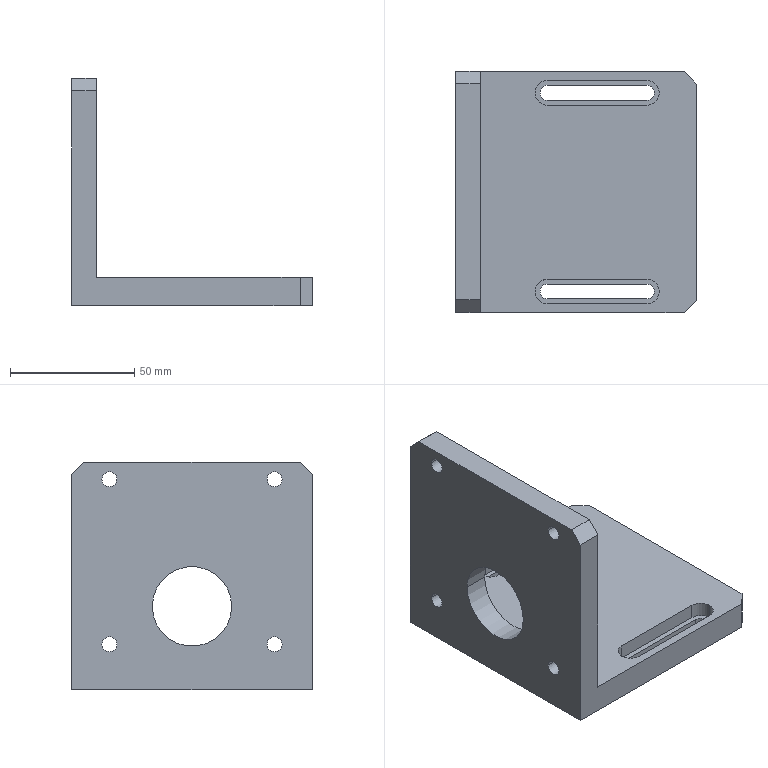Part | STEP file | Motor fixing bracket | 1 solid | 44 faces | box 97 x 97 x 91.5 mm | volume 167399 mm3 | cylinder 22 | plane 22 | commonest cylinder face diameters 6 x14 10 x6 32 x2
STEP:
#1=CARTESIAN_POINT('',(28.5,45.,5.5));
#2=VERTEX_POINT('',#1);
#3=CARTESIAN_POINT('',(33.5,40.,5.5));
#4=VERTEX_POINT('',#3);
#5=CARTESIAN_POINT('',(28.5,40.,5.5));
#6=DIRECTION('',(0.,0.,-1.));
#7=DIRECTION('',(1.,0.,0.));
#8=AXIS2_PLACEMENT_3D('',#5,#6,#7);
#9=CIRCLE('',#8,5.);
#10=EDGE_CURVE('',#2,#4,#9,.T.);
#11=ORIENTED_EDGE('',*,*,#10,.T.);
#12=CARTESIAN_POINT('',(33.5,40.,11.5));
#13=VERTEX_POINT('',#12);
#14=CARTESIAN_POINT('',(33.5,40.,5.5));
#15=DIRECTION('',(0.,0.,1.));
#16=VECTOR('',#15,1000.);
#17=LINE('',#14,#16);
#18=EDGE_CURVE('',#4,#13,#17,.T.);
#19=ORIENTED_EDGE('',*,*,#18,.T.);
#20=CARTESIAN_POINT('',(28.5,45.,11.5));
#21=VERTEX_POINT('',#20);
#22=CARTESIAN_POINT('',(28.5,40.,11.5));
#23=DIRECTION('',(0.,0.,-1.));
#24=DIRECTION('',(1.,0.,0.));
#25=AXIS2_PLACEMENT_3D('',#22,#23,#24);
#26=CIRCLE('',#25,5.);
#27=EDGE_CURVE('',#21,#13,#26,.T.);
#28=ORIENTED_EDGE('',*,*,#27,.F.);
#29=CARTESIAN_POINT('',(28.5,45.,5.5));
#30=DIRECTION('',(0.,0.,1.));
#31=VECTOR('',#30,1000.);
#32=LINE('',#29,#31);
#33=EDGE_CURVE('',#2,#21,#32,.T.);
#34=ORIENTED_EDGE('',*,*,#33,.F.);
#35=EDGE_LOOP('',(#11,#19,#28,#34));
#36=FACE_OUTER_BOUND('',#35,.T.);
#37=CARTESIAN_POINT('',(28.5,40.,5.5));
#38=DIRECTION('',(0.,0.,1.));
#39=DIRECTION('',(1.,0.,0.));
#40=AXIS2_PLACEMENT_3D('',#37,#38,#39);
#41=CYLINDRICAL_SURFACE('',#40,5.);
#42=ADVANCED_FACE('',(#36),#41,.F.);
#43=CARTESIAN_POINT('',(33.5,-40.,5.5));
#44=VERTEX_POINT('',#43);
#45=CARTESIAN_POINT('',(28.5,-35.,5.5));
#46=VERTEX_POINT('',#45);
#47=CARTESIAN_POINT('',(28.5,-40.,5.5));
#48=DIRECTION('',(0.,0.,1.));
#49=DIRECTION('',(1.,0.,0.));
#50=AXIS2_PLACEMENT_3D('',#47,#48,#49);
#51=CIRCLE('',#50,5.);
#52=EDGE_CURVE('',#44,#46,#51,.T.);
#53=ORIENTED_EDGE('',*,*,#52,.F.);
#54=CARTESIAN_POINT('',(33.5,-40.,11.5));
#55=VERTEX_POINT('',#54);
#56=CARTESIAN_POINT('',(33.5,-40.,5.5));
#57=DIRECTION('',(0.,0.,1.));
#58=VECTOR('',#57,1000.);
#59=LINE('',#56,#58);
#60=EDGE_CURVE('',#44,#55,#59,.T.);
#61=ORIENTED_EDGE('',*,*,#60,.T.);
#62=CARTESIAN_POINT('',(28.5,-35.,11.5));
#63=VERTEX_POINT('',#62);
#64=CARTESIAN_POINT('',(28.5,-40.,11.5));
#65=DIRECTION('',(0.,0.,1.));
#66=DIRECTION('',(1.,0.,0.));
#67=AXIS2_PLACEMENT_3D('',#64,#65,#66);
#68=CIRCLE('',#67,5.);
#69=EDGE_CURVE('',#55,#63,#68,.T.);
#70=ORIENTED_EDGE('',*,*,#69,.T.);
#71=CARTESIAN_POINT('',(28.5,-35.,5.5));
#72=DIRECTION('',(0.,0.,1.));
#73=VECTOR('',#72,1000.);
#74=LINE('',#71,#73);
#75=EDGE_CURVE('',#46,#63,#74,.T.);
#76=ORIENTED_EDGE('',*,*,#75,.F.);
#77=EDGE_LOOP('',(#53,#61,#70,#76));
#78=FACE_OUTER_BOUND('',#77,.T.);
#79=CARTESIAN_POINT('',(28.5,-40.,5.5));
#80=DIRECTION('',(0.,0.,1.));
#81=DIRECTION('',(1.,0.,0.));
#82=AXIS2_PLACEMENT_3D('',#79,#80,#81);
#83=CYLINDRICAL_SURFACE('',#82,5.);
#84=ADVANCED_FACE('',(#78),#83,.F.);
#85=CARTESIAN_POINT('',(-38.5,36.234,84.734));
#86=VERTEX_POINT('',#85);
#87=CARTESIAN_POINT('',(-38.5,30.234,84.734));
#88=VERTEX_POINT('',#87);
#89=CARTESIAN_POINT('',(-38.5,33.234,84.734));
#90=DIRECTION('',(-1.,0.,0.));
#91=DIRECTION('',(0.,0.,1.));
#92=AXIS2_PLACEMENT_3D('',#89,#90,#91);
#93=CIRCLE('',#92,3.);
#94=EDGE_CURVE('',#86,#88,#93,.T.);
#95=ORIENTED_EDGE('',*,*,#94,.F.);
#96=CARTESIAN_POINT('',(-48.5,36.234,84.734));
#97=VERTEX_POINT('',#96);
#98=CARTESIAN_POINT('',(31.5,36.234,84.734));
#99=DIRECTION('',(-1.,0.,0.));
#100=VECTOR('',#99,1000.);
#101=LINE('',#98,#100);
#102=EDGE_CURVE('',#86,#97,#101,.T.);
#103=ORIENTED_EDGE('',*,*,#102,.T.);
#104=CARTESIAN_POINT('',(-48.5,30.234,84.734));
#105=VERTEX_POINT('',#104);
#106=CARTESIAN_POINT('',(-48.5,33.234,84.734));
#107=DIRECTION('',(-1.,0.,0.));
#108=DIRECTION('',(0.,-1.,0.));
#109=AXIS2_PLACEMENT_3D('',#106,#107,#108);
#110=CIRCLE('',#109,3.);
#111=EDGE_CURVE('',#97,#105,#110,.T.);
#112=ORIENTED_EDGE('',*,*,#111,.T.);
#113=CARTESIAN_POINT('',(31.5,30.234,84.734));
#114=DIRECTION('',(-1.,0.,0.));
#115=VECTOR('',#114,1000.);
#116=LINE('',#113,#115);
#117=EDGE_CURVE('',#88,#105,#116,.T.);
#118=ORIENTED_EDGE('',*,*,#117,.F.);
#119=EDGE_LOOP('',(#95,#103,#112,#118));
#120=FACE_OUTER_BOUND('',#119,.T.);
#121=CARTESIAN_POINT('',(31.5,33.234,84.734));
#122=DIRECTION('',(-1.,0.,0.));
#123=DIRECTION('',(0.,-1.,0.));
#124=AXIS2_PLACEMENT_3D('',#121,#122,#123);
#125=CYLINDRICAL_SURFACE('',#124,3.);
#126=ADVANCED_FACE('',(#120),#125,.F.);
#127=CARTESIAN_POINT('',(-38.5,-30.234,84.734));
#128=VERTEX_POINT('',#127);
#129=CARTESIAN_POINT('',(-38.5,-36.234,84.734));
#130=VERTEX_POINT('',#129);
#131=CARTESIAN_POINT('',(-38.5,-33.234,84.734));
#132=DIRECTION('',(-1.,0.,0.));
#133=DIRECTION('',(0.,0.,1.));
#134=AXIS2_PLACEMENT_3D('',#131,#132,#133);
#135=CIRCLE('',#134,3.);
#136=EDGE_CURVE('',#128,#130,#135,.T.);
#137=ORIENTED_EDGE('',*,*,#136,.F.);
#138=CARTESIAN_POINT('',(-48.5,-30.234,84.734));
#139=VERTEX_POINT('',#138);
#140=CARTESIAN_POINT('',(31.5,-30.234,84.734));
#141=DIRECTION('',(-1.,0.,0.));
#142=VECTOR('',#141,1000.);
#143=LINE('',#140,#142);
#144=EDGE_CURVE('',#128,#139,#143,.T.);
#145=ORIENTED_EDGE('',*,*,#144,.T.);
#146=CARTESIAN_POINT('',(-48.5,-36.234,84.734));
#147=VERTEX_POINT('',#146);
#148=CARTESIAN_POINT('',(-48.5,-33.234,84.734));
#149=DIRECTION('',(-1.,0.,0.));
#150=DIRECTION('',(0.,1.,0.));
#151=AXIS2_PLACEMENT_3D('',#148,#149,#150);
#152=CIRCLE('',#151,3.);
#153=EDGE_CURVE('',#139,#147,#152,.T.);
#154=ORIENTED_EDGE('',*,*,#153,.T.);
#155=CARTESIAN_POINT('',(31.5,-36.234,84.734));
#156=DIRECTION('',(-1.,0.,0.));
#157=VECTOR('',#156,1000.);
#158=LINE('',#155,#157);
#159=EDGE_CURVE('',#130,#147,#158,.T.);
#160=ORIENTED_EDGE('',*,*,#159,.F.);
#161=EDGE_LOOP('',(#137,#145,#154,#160));
#162=FACE_OUTER_BOUND('',#161,.T.);
#163=CARTESIAN_POINT('',(31.5,-33.234,84.734));
#164=DIRECTION('',(-1.,0.,0.));
#165=DIRECTION('',(0.,-1.,0.));
#166=AXIS2_PLACEMENT_3D('',#163,#164,#165);
#167=CYLINDRICAL_SURFACE('',#166,3.);
#168=ADVANCED_FACE('',(#162),#167,.F.);
#169=CARTESIAN_POINT('',(-38.5,-30.234,18.266));
#170=VERTEX_POINT('',#169);
#171=CARTESIAN_POINT('',(-38.5,-36.234,18.266));
#172=VERTEX_POINT('',#171);
#173=CARTESIAN_POINT('',(-38.5,-33.234,18.266));
#174=DIRECTION('',(-1.,0.,0.));
#175=DIRECTION('',(0.,0.,1.));
#176=AXIS2_PLACEMENT_3D('',#173,#174,#175);
#177=CIRCLE('',#176,3.);
#178=EDGE_CURVE('',#170,#172,#177,.T.);
#179=ORIENTED_EDGE('',*,*,#178,.F.);
#180=CARTESIAN_POINT('',(-48.5,-30.234,18.266));
#181=VERTEX_POINT('',#180);
#182=CARTESIAN_POINT('',(31.5,-30.234,18.266));
#183=DIRECTION('',(-1.,0.,0.));
#184=VECTOR('',#183,1000.);
#185=LINE('',#182,#184);
#186=EDGE_CURVE('',#170,#181,#185,.T.);
#187=ORIENTED_EDGE('',*,*,#186,.T.);
#188=CARTESIAN_POINT('',(-48.5,-36.234,18.266));
#189=VERTEX_POINT('',#188);
#190=CARTESIAN_POINT('',(-48.5,-33.234,18.266));
#191=DIRECTION('',(-1.,0.,0.));
#192=DIRECTION('',(0.,-1.,0.));
#193=AXIS2_PLACEMENT_3D('',#190,#191,#192);
#194=CIRCLE('',#193,3.);
#195=EDGE_CURVE('',#181,#189,#194,.T.);
#196=ORIENTED_EDGE('',*,*,#195,.T.);
#197=CARTESIAN_POINT('',(31.5,-36.234,18.266));
#198=DIRECTION('',(-1.,0.,0.));
#199=VECTOR('',#198,1000.);
#200=LINE('',#197,#199);
#201=EDGE_CURVE('',#172,#189,#200,.T.);
#202=ORIENTED_EDGE('',*,*,#201,.F.);
#203=EDGE_LOOP('',(#179,#187,#196,#202));
#204=FACE_OUTER_BOUND('',#203,.T.);
#205=CARTESIAN_POINT('',(31.5,-33.234,18.266));
#206=DIRECTION('',(-1.,0.,0.));
#207=DIRECTION('',(0.,-1.,0.));
#208=AXIS2_PLACEMENT_3D('',#205,#206,#207);
#209=CYLINDRICAL_SURFACE('',#208,3.);
#210=ADVANCED_FACE('',(#204),#209,.F.);
#211=CARTESIAN_POINT('',(-38.5,36.234,18.266));
#212=VERTEX_POINT('',#211);
#213=CARTESIAN_POINT('',(-38.5,30.234,18.266));
#214=VERTEX_POINT('',#213);
#215=CARTESIAN_POINT('',(-38.5,33.234,18.266));
#216=DIRECTION('',(-1.,0.,0.));
#217=DIRECTION('',(0.,0.,1.));
#218=AXIS2_PLACEMENT_3D('',#215,#216,#217);
#219=CIRCLE('',#218,3.);
#220=EDGE_CURVE('',#212,#214,#219,.T.);
#221=ORIENTED_EDGE('',*,*,#220,.F.);
#222=CARTESIAN_POINT('',(-48.5,36.234,18.266));
#223=VERTEX_POINT('',#222);
#224=CARTESIAN_POINT('',(31.5,36.234,18.266));
#225=DIRECTION('',(-1.,0.,0.));
#226=VECTOR('',#225,1000.);
#227=LINE('',#224,#226);
#228=EDGE_CURVE('',#212,#223,#227,.T.);
#229=ORIENTED_EDGE('',*,*,#228,.T.);
#230=CARTESIAN_POINT('',(-48.5,30.234,18.266));
#231=VERTEX_POINT('',#230);
#232=CARTESIAN_POINT('',(-48.5,33.234,18.266));
#233=DIRECTION('',(-1.,0.,0.));
#234=DIRECTION('',(0.,1.,0.));
#235=AXIS2_PLACEMENT_3D('',#232,#233,#234);
#236=CIRCLE('',#235,3.);
#237=EDGE_CURVE('',#223,#231,#236,.T.);
#238=ORIENTED_EDGE('',*,*,#237,.T.);
#239=CARTESIAN_POINT('',(31.5,30.234,18.266));
#240=DIRECTION('',(-1.,0.,0.));
#241=VECTOR('',#240,1000.);
#242=LINE('',#239,#241);
#243=EDGE_CURVE('',#214,#231,#242,.T.);
#244=ORIENTED_EDGE('',*,*,#243,.F.);
#245=EDGE_LOOP('',(#221,#229,#238,#244));
#246=FACE_OUTER_BOUND('',#245,.T.);
#247=CARTESIAN_POINT('',(31.5,33.234,18.266));
#248=DIRECTION('',(-1.,0.,0.));
#249=DIRECTION('',(0.,-1.,0.));
#250=AXIS2_PLACEMENT_3D('',#247,#248,#249);
#251=CYLINDRICAL_SURFACE('',#250,3.);
#252=ADVANCED_FACE('',(#246),#251,.F.);
#253=CARTESIAN_POINT('',(-38.5,16.,33.5));
#254=VERTEX_POINT('',#253);
#255=CARTESIAN_POINT('',(-38.5,-16.,33.5));
#256=VERTEX_POINT('',#255);
#257=CARTESIAN_POINT('',(-38.5,0.,33.5));
#258=DIRECTION('',(-1.,0.,0.));
#259=DIRECTION('',(0.,0.,1.));
#260=AXIS2_PLACEMENT_3D('',#257,#258,#259);
#261=CIRCLE('',#260,16.);
#262=EDGE_CURVE('',#254,#256,#261,.T.);
#263=ORIENTED_EDGE('',*,*,#262,.F.);
#264=CARTESIAN_POINT('',(-48.5,16.,33.5));
#265=VERTEX_POINT('',#264);
#266=CARTESIAN_POINT('',(31.5,16.,33.5));
#267=DIRECTION('',(-1.,0.,0.));
#268=VECTOR('',#267,1000.);
#269=LINE('',#266,#268);
#270=EDGE_CURVE('',#254,#265,#269,.T.);
#271=ORIENTED_EDGE('',*,*,#270,.T.);
#272=CARTESIAN_POINT('',(-48.5,-16.,33.5));
#273=VERTEX_POINT('',#272);
#274=CARTESIAN_POINT('',(-48.5,0.,33.5));
#275=DIRECTION('',(-1.,0.,0.));
#276=DIRECTION('',(0.,-1.,0.));
#277=AXIS2_PLACEMENT_3D('',#274,#275,#276);
#278=CIRCLE('',#277,16.);
#279=EDGE_CURVE('',#265,#273,#278,.T.);
#280=ORIENTED_EDGE('',*,*,#279,.T.);
#281=CARTESIAN_POINT('',(31.5,-16.,33.5));
#282=DIRECTION('',(-1.,0.,0.));
#283=VECTOR('',#282,1000.);
#284=LINE('',#281,#283);
#285=EDGE_CURVE('',#256,#273,#284,.T.);
#286=ORIENTED_EDGE('',*,*,#285,.F.);
#287=EDGE_LOOP('',(#263,#271,#280,#286));
#288=FACE_OUTER_BOUND('',#287,.T.);
#289=CARTESIAN_POINT('',(31.5,0.,33.5));
#290=DIRECTION('',(-1.,0.,0.));
#291=DIRECTION('',(0.,-1.,0.));
#292=AXIS2_PLACEMENT_3D('',#289,#290,#291);
#293=CYLINDRICAL_SURFACE('',#292,16.);
#294=ADVANCED_FACE('',(#288),#293,.F.);
#295=CARTESIAN_POINT('',(31.5,-40.,0.));
#296=VERTEX_POINT('',#295);
#297=CARTESIAN_POINT('',(28.5,-37.,0.));
#298=VERTEX_POINT('',#297);
#299=CARTESIAN_POINT('',(28.5,-40.,0.));
#300=DIRECTION('',(0.,0.,1.));
#301=DIRECTION('',(1.,0.,0.));
#302=AXIS2_PLACEMENT_3D('',#299,#300,#301);
#303=CIRCLE('',#302,3.);
#304=EDGE_CURVE('',#296,#298,#303,.T.);
#305=ORIENTED_EDGE('',*,*,#304,.F.);
#306=CARTESIAN_POINT('',(31.5,-40.,5.5));
#307=VERTEX_POINT('',#306);
#308=CARTESIAN_POINT('',(31.5,-40.,-8.5));
#309=DIRECTION('',(0.,0.,1.));
#310=VECTOR('',#309,1000.);
#311=LINE('',#308,#310);
#312=EDGE_CURVE('',#296,#307,#311,.T.);
#313=ORIENTED_EDGE('',*,*,#312,.T.);
#314=CARTESIAN_POINT('',(28.5,-37.,5.5));
#315=VERTEX_POINT('',#314);
#316=CARTESIAN_POINT('',(28.5,-40.,5.5));
#317=DIRECTION('',(0.,0.,-1.));
#318=DIRECTION('',(1.,0.,0.));
#319=AXIS2_PLACEMENT_3D('',#316,#317,#318);
#320=CIRCLE('',#319,3.);
#321=EDGE_CURVE('',#315,#307,#320,.T.);
#322=ORIENTED_EDGE('',*,*,#321,.F.);
#323=CARTESIAN_POINT('',(28.5,-37.,-8.5));
#324=DIRECTION('',(0.,0.,1.));
#325=VECTOR('',#324,1000.);
#326=LINE('',#323,#325);
#327=EDGE_CURVE('',#298,#315,#326,.T.);
#328=ORIENTED_EDGE('',*,*,#327,.F.);
#329=EDGE_LOOP('',(#305,#313,#322,#328));
#330=FACE_OUTER_BOUND('',#329,.T.);
#331=CARTESIAN_POINT('',(28.5,-40.,-8.5));
#332=DIRECTION('',(0.,0.,1.));
#333=DIRECTION('',(1.,0.,0.));
#334=AXIS2_PLACEMENT_3D('',#331,#332,#333);
#335=CYLINDRICAL_SURFACE('',#334,3.);
#336=ADVANCED_FACE('',(#330),#335,.F.);
#337=CARTESIAN_POINT('',(28.5,43.,0.));
#338=VERTEX_POINT('',#337);
#339=CARTESIAN_POINT('',(31.5,40.,0.));
#340=VERTEX_POINT('',#339);
#341=CARTESIAN_POINT('',(28.5,40.,0.));
#342=DIRECTION('',(0.,0.,-1.));
#343=DIRECTION('',(1.,0.,0.));
#344=AXIS2_PLACEMENT_3D('',#341,#342,#343);
#345=CIRCLE('',#344,3.);
#346=EDGE_CURVE('',#338,#340,#345,.T.);
#347=ORIENTED_EDGE('',*,*,#346,.T.);
#348=CARTESIAN_POINT('',(31.5,40.,5.5));
#349=VERTEX_POINT('',#348);
#350=CARTESIAN_POINT('',(31.5,40.,-8.5));
#351=DIRECTION('',(0.,0.,1.));
#352=VECTOR('',#351,1000.);
#353=LINE('',#350,#352);
#354=EDGE_CURVE('',#340,#349,#353,.T.);
#355=ORIENTED_EDGE('',*,*,#354,.T.);
#356=CARTESIAN_POINT('',(28.5,43.,5.5));
#357=VERTEX_POINT('',#356);
#358=CARTESIAN_POINT('',(28.5,40.,5.5));
#359=DIRECTION('',(0.,0.,1.));
#360=DIRECTION('',(1.,0.,0.));
#361=AXIS2_PLACEMENT_3D('',#358,#359,#360);
#362=CIRCLE('',#361,3.);
#363=EDGE_CURVE('',#349,#357,#362,.T.);
#364=ORIENTED_EDGE('',*,*,#363,.T.);
#365=CARTESIAN_POINT('',(28.5,43.,-8.5));
#366=DIRECTION('',(0.,0.,1.));
#367=VECTOR('',#366,1000.);
#368=LINE('',#365,#367);
#369=EDGE_CURVE('',#338,#357,#368,.T.);
#370=ORIENTED_EDGE('',*,*,#369,.F.);
#371=EDGE_LOOP('',(#347,#355,#364,#370));
#372=FACE_OUTER_BOUND('',#371,.T.);
#373=CARTESIAN_POINT('',(28.5,40.,-8.5));
#374=DIRECTION('',(0.,0.,1.));
#375=DIRECTION('',(1.,0.,0.));
#376=AXIS2_PLACEMENT_3D('',#373,#374,#375);
#377=CYLINDRICAL_SURFACE('',#376,3.);
#378=ADVANCED_FACE('',(#372),#377,.F.);
#379=CARTESIAN_POINT('',(48.5,-43.5,11.5));
#380=VERTEX_POINT('',#379);
#381=CARTESIAN_POINT('',(48.5,43.5,11.5));
#382=VERTEX_POINT('',#381);
#383=CARTESIAN_POINT('',(48.5,48.5,11.5));
#384=DIRECTION('',(0.,1.,0.));
#385=VECTOR('',#384,1000.);
#386=LINE('',#383,#385);
#387=EDGE_CURVE('',#380,#382,#386,.T.);
#388=ORIENTED_EDGE('',*,*,#387,.T.);
#389=CARTESIAN_POINT('',(43.5,48.5,11.5));
#390=VERTEX_POINT('',#389);
#391=CARTESIAN_POINT('',(46.,46.,11.5));
#392=DIRECTION('',(-0.7071,0.7071,0.));
#393=VECTOR('',#392,1000.);
#394=LINE('',#391,#393);
#395=EDGE_CURVE('',#382,#390,#394,.T.);
#396=ORIENTED_EDGE('',*,*,#395,.T.);
#397=CARTESIAN_POINT('',(-38.5,48.5,11.5));
#398=VERTEX_POINT('',#397);
#399=CARTESIAN_POINT('',(-48.5,48.5,11.5));
#400=DIRECTION('',(-1.,0.,0.));
#401=VECTOR('',#400,1000.);
#402=LINE('',#399,#401);
#403=EDGE_CURVE('',#390,#398,#402,.T.);
#404=ORIENTED_EDGE('',*,*,#403,.T.);
#405=CARTESIAN_POINT('',(-38.5,-48.5,11.5));
#406=VERTEX_POINT('',#405);
#407=CARTESIAN_POINT('',(-38.5,-48.5,11.5));
#408=DIRECTION('',(0.,1.,0.));
#409=VECTOR('',#408,1000.);
#410=LINE('',#407,#409);
#411=EDGE_CURVE('',#406,#398,#410,.T.);
#412=ORIENTED_EDGE('',*,*,#411,.F.);
#413=CARTESIAN_POINT('',(43.5,-48.5,11.5));
#414=VERTEX_POINT('',#413);
#415=CARTESIAN_POINT('',(-48.5,-48.5,11.5));
#416=DIRECTION('',(1.,0.,0.));
#417=VECTOR('',#416,1000.);
#418=LINE('',#415,#417);
#419=EDGE_CURVE('',#406,#414,#418,.T.);
#420=ORIENTED_EDGE('',*,*,#419,.T.);
#421=CARTESIAN_POINT('',(46.,-46.,11.5));
#422=DIRECTION('',(0.7071,0.7071,0.));
#423=VECTOR('',#422,1000.);
#424=LINE('',#421,#423);
#425=EDGE_CURVE('',#414,#380,#424,.T.);
#426=ORIENTED_EDGE('',*,*,#425,.T.);
#427=EDGE_LOOP('',(#388,#396,#404,#412,#420,#426));
#428=FACE_OUTER_BOUND('',#427,.T.);
#429=CARTESIAN_POINT('',(-11.5,-35.,11.5));
#430=VERTEX_POINT('',#429);
#431=CARTESIAN_POINT('',(-11.5,-45.,11.5));
#432=VERTEX_POINT('',#431);
#433=CARTESIAN_POINT('',(-11.5,-40.,11.5));
#434=DIRECTION('',(0.,0.,1.));
#435=DIRECTION('',(1.,0.,0.));
#436=AXIS2_PLACEMENT_3D('',#433,#434,#435);
#437=CIRCLE('',#436,5.);
#438=EDGE_CURVE('',#430,#432,#437,.T.);
#439=ORIENTED_EDGE('',*,*,#438,.F.);
#440=CARTESIAN_POINT('',(-11.5,-35.,11.5));
#441=DIRECTION('',(-1.,0.,0.));
#442=VECTOR('',#441,1000.);
#443=LINE('',#440,#442);
#444=EDGE_CURVE('',#63,#430,#443,.T.);
#445=ORIENTED_EDGE('',*,*,#444,.F.);
#446=ORIENTED_EDGE('',*,*,#69,.F.);
#447=CARTESIAN_POINT('',(28.5,-45.,11.5));
#448=VERTEX_POINT('',#447);
#449=CARTESIAN_POINT('',(28.5,-40.,11.5));
#450=DIRECTION('',(0.,0.,1.));
#451=DIRECTION('',(1.,0.,0.));
#452=AXIS2_PLACEMENT_3D('',#449,#450,#451);
#453=CIRCLE('',#452,5.);
#454=EDGE_CURVE('',#448,#55,#453,.T.);
#455=ORIENTED_EDGE('',*,*,#454,.F.);
#456=CARTESIAN_POINT('',(-11.5,-45.,11.5));
#457=DIRECTION('',(1.,0.,0.));
#458=VECTOR('',#457,1000.);
#459=LINE('',#456,#458);
#460=EDGE_CURVE('',#432,#448,#459,.T.);
#461=ORIENTED_EDGE('',*,*,#460,.F.);
#462=EDGE_LOOP('',(#439,#445,#446,#455,#461));
#463=FACE_BOUND('',#462,.T.);
#464=CARTESIAN_POINT('',(28.5,35.,11.5));
#465=VERTEX_POINT('',#464);
#466=CARTESIAN_POINT('',(-11.5,35.,11.5));
#467=VERTEX_POINT('',#466);
#468=CARTESIAN_POINT('',(-11.5,35.,11.5));
#469=DIRECTION('',(-1.,0.,0.));
#470=VECTOR('',#469,1000.);
#471=LINE('',#468,#470);
#472=EDGE_CURVE('',#465,#467,#471,.T.);
#473=ORIENTED_EDGE('',*,*,#472,.T.);
#474=CARTESIAN_POINT('',(-11.5,45.,11.5));
#475=VERTEX_POINT('',#474);
#476=CARTESIAN_POINT('',(-11.5,40.,11.5));
#477=DIRECTION('',(0.,0.,-1.));
#478=DIRECTION('',(1.,0.,0.));
#479=AXIS2_PLACEMENT_3D('',#476,#477,#478);
#480=CIRCLE('',#479,5.);
#481=EDGE_CURVE('',#467,#475,#480,.T.);
#482=ORIENTED_EDGE('',*,*,#481,.T.);
#483=CARTESIAN_POINT('',(-11.5,45.,11.5));
#484=DIRECTION('',(1.,0.,0.));
#485=VECTOR('',#484,1000.);
#486=LINE('',#483,#485);
#487=EDGE_CURVE('',#475,#21,#486,.T.);
#488=ORIENTED_EDGE('',*,*,#487,.T.);
#489=ORIENTED_EDGE('',*,*,#27,.T.);
#490=CARTESIAN_POINT('',(28.5,40.,11.5));
#491=DIRECTION('',(0.,0.,-1.));
#492=DIRECTION('',(1.,0.,0.));
#493=AXIS2_PLACEMENT_3D('',#490,#491,#492);
#494=CIRCLE('',#493,5.);
#495=EDGE_CURVE('',#13,#465,#494,.T.);
#496=ORIENTED_EDGE('',*,*,#495,.T.);
#497=EDGE_LOOP('',(#473,#482,#488,#489,#496));
#498=FACE_BOUND('',#497,.T.);
#499=CARTESIAN_POINT('',(0.,0.,11.5));
#500=DIRECTION('',(0.,0.,1.));
#501=DIRECTION('',(1.,0.,0.));
#502=AXIS2_PLACEMENT_3D('',#499,#500,#501);
#503=PLANE('',#502);
#504=ADVANCED_FACE('',(#428,#463,#498),#503,.T.);
#505=CARTESIAN_POINT('',(-11.5,43.,0.));
#506=VERTEX_POINT('',#505);
#507=CARTESIAN_POINT('',(-11.5,43.,5.5));
#508=VERTEX_POINT('',#507);
#509=CARTESIAN_POINT('',(-11.5,43.,-8.5));
#510=DIRECTION('',(0.,0.,1.));
#511=VECTOR('',#510,1000.);
#512=LINE('',#509,#511);
#513=EDGE_CURVE('',#506,#508,#512,.T.);
#514=ORIENTED_EDGE('',*,*,#513,.T.);
#515=CARTESIAN_POINT('',(-11.5,37.,5.5));
#516=VERTEX_POINT('',#515);
#517=CARTESIAN_POINT('',(-11.5,40.,5.5));
#518=DIRECTION('',(0.,0.,1.));
#519=DIRECTION('',(1.,0.,0.));
#520=AXIS2_PLACEMENT_3D('',#517,#518,#519);
#521=CIRCLE('',#520,3.);
#522=EDGE_CURVE('',#508,#516,#521,.T.);
#523=ORIENTED_EDGE('',*,*,#522,.T.);
#524=CARTESIAN_POINT('',(-11.5,37.,0.));
#525=VERTEX_POINT('',#524);
#526=CARTESIAN_POINT('',(-11.5,37.,-8.5));
#527=DIRECTION('',(0.,0.,1.));
#528=VECTOR('',#527,1000.);
#529=LINE('',#526,#528);
#530=EDGE_CURVE('',#525,#516,#529,.T.);
#531=ORIENTED_EDGE('',*,*,#530,.F.);
#532=CARTESIAN_POINT('',(-11.5,40.,0.));
#533=DIRECTION('',(0.,0.,-1.));
#534=DIRECTION('',(1.,0.,0.));
#535=AXIS2_PLACEMENT_3D('',#532,#533,#534);
#536=CIRCLE('',#535,3.);
#537=EDGE_CURVE('',#525,#506,#536,.T.);
#538=ORIENTED_EDGE('',*,*,#537,.T.);
#539=EDGE_LOOP('',(#514,#523,#531,#538));
#540=FACE_OUTER_BOUND('',#539,.T.);
#541=CARTESIAN_POINT('',(-11.5,40.,-8.5));
#542=DIRECTION('',(0.,0.,1.));
#543=DIRECTION('',(1.,0.,0.));
#544=AXIS2_PLACEMENT_3D('',#541,#542,#543);
#545=CYLINDRICAL_SURFACE('',#544,3.);
#546=ADVANCED_FACE('',(#540),#545,.F.);
#547=ORIENTED_EDGE('',*,*,#369,.T.);
#548=CARTESIAN_POINT('',(-11.5,43.,5.5));
#549=DIRECTION('',(-1.,0.,0.));
#550=VECTOR('',#549,1000.);
#551=LINE('',#548,#550);
#552=EDGE_CURVE('',#357,#508,#551,.T.);
#553=ORIENTED_EDGE('',*,*,#552,.T.);
#554=ORIENTED_EDGE('',*,*,#513,.F.);
#555=CARTESIAN_POINT('',(0.,43.,0.));
#556=DIRECTION('',(1.,0.,0.));
#557=VECTOR('',#556,1000.);
#558=LINE('',#555,#557);
#559=EDGE_CURVE('',#506,#338,#558,.T.);
#560=ORIENTED_EDGE('',*,*,#559,.T.);
#561=EDGE_LOOP('',(#547,#553,#554,#560));
#562=FACE_OUTER_BOUND('',#561,.T.);
#563=CARTESIAN_POINT('',(-11.5,43.,-8.5));
#564=DIRECTION('',(0.,-1.,0.));
#565=DIRECTION('',(1.,0.,0.));
#566=AXIS2_PLACEMENT_3D('',#563,#564,#565);
#567=PLANE('',#566);
#568=ADVANCED_FACE('',(#562),#567,.T.);
#569=ORIENTED_EDGE('',*,*,#354,.F.);
#570=CARTESIAN_POINT('',(28.5,37.,0.));
#571=VERTEX_POINT('',#570);
#572=CARTESIAN_POINT('',(28.5,40.,0.));
#573=DIRECTION('',(0.,0.,-1.));
#574=DIRECTION('',(1.,0.,0.));
#575=AXIS2_PLACEMENT_3D('',#572,#573,#574);
#576=CIRCLE('',#575,3.);
#577=EDGE_CURVE('',#340,#571,#576,.T.);
#578=ORIENTED_EDGE('',*,*,#577,.T.);
#579=CARTESIAN_POINT('',(28.5,37.,5.5));
#580=VERTEX_POINT('',#579);
#581=CARTESIAN_POINT('',(28.5,37.,-8.5));
#582=DIRECTION('',(0.,0.,1.));
#583=VECTOR('',#582,1000.);
#584=LINE('',#581,#583);
#585=EDGE_CURVE('',#571,#580,#584,.T.);
#586=ORIENTED_EDGE('',*,*,#585,.T.);
#587=CARTESIAN_POINT('',(28.5,40.,5.5));
#588=DIRECTION('',(0.,0.,1.));
#589=DIRECTION('',(1.,0.,0.));
#590=AXIS2_PLACEMENT_3D('',#587,#588,#589);
#591=CIRCLE('',#590,3.);
#592=EDGE_CURVE('',#580,#349,#591,.T.);
#593=ORIENTED_EDGE('',*,*,#592,.T.);
#594=EDGE_LOOP('',(#569,#578,#586,#593));
#595=FACE_OUTER_BOUND('',#594,.T.);
#596=CARTESIAN_POINT('',(28.5,40.,-8.5));
#597=DIRECTION('',(0.,0.,1.));
#598=DIRECTION('',(1.,0.,0.));
#599=AXIS2_PLACEMENT_3D('',#596,#597,#598);
#600=CYLINDRICAL_SURFACE('',#599,3.);
#601=ADVANCED_FACE('',(#595),#600,.F.);
#602=ORIENTED_EDGE('',*,*,#530,.T.);
#603=CARTESIAN_POINT('',(-11.5,37.,5.5));
#604=DIRECTION('',(1.,0.,0.));
#605=VECTOR('',#604,1000.);
#606=LINE('',#603,#605);
#607=EDGE_CURVE('',#516,#580,#606,.T.);
#608=ORIENTED_EDGE('',*,*,#607,.T.);
#609=ORIENTED_EDGE('',*,*,#585,.F.);
#610=CARTESIAN_POINT('',(0.,37.,0.));
#611=DIRECTION('',(-1.,0.,0.));
#612=VECTOR('',#611,1000.);
#613=LINE('',#610,#612);
#614=EDGE_CURVE('',#571,#525,#613,.T.);
#615=ORIENTED_EDGE('',*,*,#614,.T.);
#616=EDGE_LOOP('',(#602,#608,#609,#615));
#617=FACE_OUTER_BOUND('',#616,.T.);
#618=CARTESIAN_POINT('',(-11.5,37.,-8.5));
#619=DIRECTION('',(0.,1.,0.));
#620=DIRECTION('',(-1.,0.,0.));
#621=AXIS2_PLACEMENT_3D('',#618,#619,#620);
#622=PLANE('',#621);
#623=ADVANCED_FACE('',(#617),#622,.T.);
#624=CARTESIAN_POINT('',(-11.5,-43.,5.5));
#625=VERTEX_POINT('',#624);
#626=CARTESIAN_POINT('',(-11.5,-37.,5.5));
#627=VERTEX_POINT('',#626);
#628=CARTESIAN_POINT('',(-11.5,-40.,5.5));
#629=DIRECTION('',(0.,0.,-1.));
#630=DIRECTION('',(1.,0.,0.));
#631=AXIS2_PLACEMENT_3D('',#628,#629,#630);
#632=CIRCLE('',#631,3.);
#633=EDGE_CURVE('',#625,#627,#632,.T.);
#634=ORIENTED_EDGE('',*,*,#633,.F.);
#635=CARTESIAN_POINT('',(-11.5,-43.,0.));
#636=VERTEX_POINT('',#635);
#637=CARTESIAN_POINT('',(-11.5,-43.,-8.5));
#638=DIRECTION('',(0.,0.,1.));
#639=VECTOR('',#638,1000.);
#640=LINE('',#637,#639);
#641=EDGE_CURVE('',#636,#625,#640,.T.);
#642=ORIENTED_EDGE('',*,*,#641,.F.);
#643=CARTESIAN_POINT('',(-11.5,-37.,0.));
#644=VERTEX_POINT('',#643);
#645=CARTESIAN_POINT('',(-11.5,-40.,0.));
#646=DIRECTION('',(0.,0.,1.));
#647=DIRECTION('',(1.,0.,0.));
#648=AXIS2_PLACEMENT_3D('',#645,#646,#647);
#649=CIRCLE('',#648,3.);
#650=EDGE_CURVE('',#644,#636,#649,.T.);
#651=ORIENTED_EDGE('',*,*,#650,.F.);
#652=CARTESIAN_POINT('',(-11.5,-37.,-8.5));
#653=DIRECTION('',(0.,0.,1.));
#654=VECTOR('',#653,1000.);
#655=LINE('',#652,#654);
#656=EDGE_CURVE('',#644,#627,#655,.T.);
#657=ORIENTED_EDGE('',*,*,#656,.T.);
#658=EDGE_LOOP('',(#634,#642,#651,#657));
#659=FACE_OUTER_BOUND('',#658,.T.);
#660=CARTESIAN_POINT('',(-11.5,-40.,-8.5));
#661=DIRECTION('',(0.,0.,1.));
#662=DIRECTION('',(1.,0.,0.));
#663=AXIS2_PLACEMENT_3D('',#660,#661,#662);
#664=CYLINDRICAL_SURFACE('',#663,3.);
#665=ADVANCED_FACE('',(#659),#664,.F.);
#666=CARTESIAN_POINT('',(-11.5,-37.,5.5));
#667=DIRECTION('',(1.,0.,0.));
#668=VECTOR('',#667,1000.);
#669=LINE('',#666,#668);
#670=EDGE_CURVE('',#627,#315,#669,.T.);
#671=ORIENTED_EDGE('',*,*,#670,.F.);
#672=ORIENTED_EDGE('',*,*,#656,.F.);
#673=CARTESIAN_POINT('',(0.,-37.,0.));
#674=DIRECTION('',(-1.,0.,0.));
#675=VECTOR('',#674,1000.);
#676=LINE('',#673,#675);
#677=EDGE_CURVE('',#298,#644,#676,.T.);
#678=ORIENTED_EDGE('',*,*,#677,.F.);
#679=ORIENTED_EDGE('',*,*,#327,.T.);
#680=EDGE_LOOP('',(#671,#672,#678,#679));
#681=FACE_OUTER_BOUND('',#680,.T.);
#682=CARTESIAN_POINT('',(-11.5,-37.,-8.5));
#683=DIRECTION('',(0.,1.,0.));
#684=DIRECTION('',(-1.,0.,0.));
#685=AXIS2_PLACEMENT_3D('',#682,#683,#684);
#686=PLANE('',#685);
#687=ADVANCED_FACE('',(#681),#686,.F.);
#688=ORIENTED_EDGE('',*,*,#312,.F.);
#689=CARTESIAN_POINT('',(28.5,-43.,0.));
#690=VERTEX_POINT('',#689);
#691=CARTESIAN_POINT('',(28.5,-40.,0.));
#692=DIRECTION('',(0.,0.,1.));
#693=DIRECTION('',(1.,0.,0.));
#694=AXIS2_PLACEMENT_3D('',#691,#692,#693);
#695=CIRCLE('',#694,3.);
#696=EDGE_CURVE('',#690,#296,#695,.T.);
#697=ORIENTED_EDGE('',*,*,#696,.F.);
#698=CARTESIAN_POINT('',(28.5,-43.,5.5));
#699=VERTEX_POINT('',#698);
#700=CARTESIAN_POINT('',(28.5,-43.,-8.5));
#701=DIRECTION('',(0.,0.,1.));
#702=VECTOR('',#701,1000.);
#703=LINE('',#700,#702);
#704=EDGE_CURVE('',#690,#699,#703,.T.);
#705=ORIENTED_EDGE('',*,*,#704,.T.);
#706=CARTESIAN_POINT('',(28.5,-40.,5.5));
#707=DIRECTION('',(0.,0.,-1.));
#708=DIRECTION('',(1.,0.,0.));
#709=AXIS2_PLACEMENT_3D('',#706,#707,#708);
#710=CIRCLE('',#709,3.);
#711=EDGE_CURVE('',#307,#699,#710,.T.);
#712=ORIENTED_EDGE('',*,*,#711,.F.);
#713=EDGE_LOOP('',(#688,#697,#705,#712));
#714=FACE_OUTER_BOUND('',#713,.T.);
#715=CARTESIAN_POINT('',(28.5,-40.,-8.5));
#716=DIRECTION('',(0.,0.,1.));
#717=DIRECTION('',(1.,0.,0.));
#718=AXIS2_PLACEMENT_3D('',#715,#716,#717);
#719=CYLINDRICAL_SURFACE('',#718,3.);
#720=ADVANCED_FACE('',(#714),#719,.F.);
#721=CARTESIAN_POINT('',(-11.5,-43.,5.5));
#722=DIRECTION('',(-1.,0.,0.));
#723=VECTOR('',#722,1000.);
#724=LINE('',#721,#723);
#725=EDGE_CURVE('',#699,#625,#724,.T.);
#726=ORIENTED_EDGE('',*,*,#725,.F.);
#727=ORIENTED_EDGE('',*,*,#704,.F.);
#728=CARTESIAN_POINT('',(0.,-43.,0.));
#729=DIRECTION('',(1.,0.,0.));
#730=VECTOR('',#729,1000.);
#731=LINE('',#728,#730);
#732=EDGE_CURVE('',#636,#690,#731,.T.);
#733=ORIENTED_EDGE('',*,*,#732,.F.);
#734=ORIENTED_EDGE('',*,*,#641,.T.);
#735=EDGE_LOOP('',(#726,#727,#733,#734));
#736=FACE_OUTER_BOUND('',#735,.T.);
#737=CARTESIAN_POINT('',(-11.5,-43.,-8.5));
#738=DIRECTION('',(0.,-1.,0.));
#739=DIRECTION('',(1.,0.,0.));
#740=AXIS2_PLACEMENT_3D('',#737,#738,#739);
#741=PLANE('',#740);
#742=ADVANCED_FACE('',(#736),#741,.F.);
#743=CARTESIAN_POINT('',(43.5,48.5,0.));
#744=VERTEX_POINT('',#743);
#745=CARTESIAN_POINT('',(-48.5,48.5,0.));
#746=VERTEX_POINT('',#745);
#747=CARTESIAN_POINT('',(-48.5,48.5,0.));
#748=DIRECTION('',(-1.,0.,0.));
#749=VECTOR('',#748,1000.);
#750=LINE('',#747,#749);
#751=EDGE_CURVE('',#744,#746,#750,.T.);
#752=ORIENTED_EDGE('',*,*,#751,.F.);
#753=CARTESIAN_POINT('',(48.5,43.5,0.));
#754=VERTEX_POINT('',#753);
#755=CARTESIAN_POINT('',(43.5,48.5,0.));
#756=DIRECTION('',(0.7071,-0.7071,0.));
#757=VECTOR('',#756,1000.);
#758=LINE('',#755,#757);
#759=EDGE_CURVE('',#744,#754,#758,.T.);
#760=ORIENTED_EDGE('',*,*,#759,.T.);
#761=CARTESIAN_POINT('',(48.5,-43.5,0.));
#762=VERTEX_POINT('',#761);
#763=CARTESIAN_POINT('',(48.5,48.5,0.));
#764=DIRECTION('',(0.,1.,0.));
#765=VECTOR('',#764,1000.);
#766=LINE('',#763,#765);
#767=EDGE_CURVE('',#762,#754,#766,.T.);
#768=ORIENTED_EDGE('',*,*,#767,.F.);
#769=CARTESIAN_POINT('',(43.5,-48.5,0.));
#770=VERTEX_POINT('',#769);
#771=CARTESIAN_POINT('',(48.5,-43.5,0.));
#772=DIRECTION('',(-0.7071,-0.7071,0.));
#773=VECTOR('',#772,1000.);
#774=LINE('',#771,#773);
#775=EDGE_CURVE('',#762,#770,#774,.T.);
#776=ORIENTED_EDGE('',*,*,#775,.T.);
#777=CARTESIAN_POINT('',(-48.5,-48.5,0.));
#778=VERTEX_POINT('',#777);
#779=CARTESIAN_POINT('',(-48.5,-48.5,0.));
#780=DIRECTION('',(1.,0.,0.));
#781=VECTOR('',#780,1000.);
#782=LINE('',#779,#781);
#783=EDGE_CURVE('',#778,#770,#782,.T.);
#784=ORIENTED_EDGE('',*,*,#783,.F.);
#785=CARTESIAN_POINT('',(-48.5,48.5,0.));
#786=DIRECTION('',(0.,-1.,0.));
#787=VECTOR('',#786,1000.);
#788=LINE('',#785,#787);
#789=EDGE_CURVE('',#746,#778,#788,.T.);
#790=ORIENTED_EDGE('',*,*,#789,.F.);
#791=EDGE_LOOP('',(#752,#760,#768,#776,#784,#790));
#792=FACE_OUTER_BOUND('',#791,.T.);
#793=ORIENTED_EDGE('',*,*,#677,.T.);
#794=ORIENTED_EDGE('',*,*,#650,.T.);
#795=ORIENTED_EDGE('',*,*,#732,.T.);
#796=ORIENTED_EDGE('',*,*,#696,.T.);
#797=ORIENTED_EDGE('',*,*,#304,.T.);
#798=EDGE_LOOP('',(#793,#794,#795,#796,#797));
#799=FACE_BOUND('',#798,.T.);
#800=ORIENTED_EDGE('',*,*,#537,.F.);
#801=ORIENTED_EDGE('',*,*,#614,.F.);
#802=ORIENTED_EDGE('',*,*,#577,.F.);
#803=ORIENTED_EDGE('',*,*,#346,.F.);
#804=ORIENTED_EDGE('',*,*,#559,.F.);
#805=EDGE_LOOP('',(#800,#801,#802,#803,#804));
#806=FACE_BOUND('',#805,.T.);
#807=CARTESIAN_POINT('',(0.,0.,0.));
#808=DIRECTION('',(0.,0.,1.));
#809=DIRECTION('',(1.,0.,0.));
#810=AXIS2_PLACEMENT_3D('',#807,#808,#809);
#811=PLANE('',#810);
#812=ADVANCED_FACE('',(#792,#799,#806),#811,.F.);
#813=ORIENTED_EDGE('',*,*,#767,.T.);
#814=CARTESIAN_POINT('',(48.5,43.5,11.5));
#815=DIRECTION('',(0.,0.,1.));
#816=VECTOR('',#815,1000.);
#817=LINE('',#814,#816);
#818=EDGE_CURVE('',#754,#382,#817,.T.);
#819=ORIENTED_EDGE('',*,*,#818,.T.);
#820=ORIENTED_EDGE('',*,*,#387,.F.);
#821=CARTESIAN_POINT('',(48.5,-43.5,11.5));
#822=DIRECTION('',(0.,0.,-1.));
#823=VECTOR('',#822,1000.);
#824=LINE('',#821,#823);
#825=EDGE_CURVE('',#380,#762,#824,.T.);
#826=ORIENTED_EDGE('',*,*,#825,.T.);
#827=EDGE_LOOP('',(#813,#819,#820,#826));
#828=FACE_OUTER_BOUND('',#827,.T.);
#829=CARTESIAN_POINT('',(48.5,48.5,11.5));
#830=DIRECTION('',(-1.,0.,0.));
#831=DIRECTION('',(0.,-1.,0.));
#832=AXIS2_PLACEMENT_3D('',#829,#830,#831);
#833=PLANE('',#832);
#834=ADVANCED_FACE('',(#828),#833,.F.);
#835=ORIENTED_EDGE('',*,*,#403,.F.);
#836=CARTESIAN_POINT('',(43.5,48.5,11.5));
#837=DIRECTION('',(0.,0.,-1.));
#838=VECTOR('',#837,1000.);
#839=LINE('',#836,#838);
#840=EDGE_CURVE('',#390,#744,#839,.T.);
#841=ORIENTED_EDGE('',*,*,#840,.T.);
#842=ORIENTED_EDGE('',*,*,#751,.T.);
#843=CARTESIAN_POINT('',(-48.5,48.5,86.5));
#844=VERTEX_POINT('',#843);
#845=CARTESIAN_POINT('',(-48.5,48.5,11.5));
#846=DIRECTION('',(0.,0.,-1.));
#847=VECTOR('',#846,1000.);
#848=LINE('',#845,#847);
#849=EDGE_CURVE('',#844,#746,#848,.T.);
#850=ORIENTED_EDGE('',*,*,#849,.F.);
#851=CARTESIAN_POINT('',(-38.5,48.5,86.5));
#852=VERTEX_POINT('',#851);
#853=CARTESIAN_POINT('',(-48.5,48.5,86.5));
#854=DIRECTION('',(1.,0.,0.));
#855=VECTOR('',#854,1000.);
#856=LINE('',#853,#855);
#857=EDGE_CURVE('',#844,#852,#856,.T.);
#858=ORIENTED_EDGE('',*,*,#857,.T.);
#859=CARTESIAN_POINT('',(-38.5,48.5,91.5));
#860=DIRECTION('',(0.,0.,-1.));
#861=VECTOR('',#860,1000.);
#862=LINE('',#859,#861);
#863=EDGE_CURVE('',#852,#398,#862,.T.);
#864=ORIENTED_EDGE('',*,*,#863,.T.);
#865=EDGE_LOOP('',(#835,#841,#842,#850,#858,#864));
#866=FACE_OUTER_BOUND('',#865,.T.);
#867=CARTESIAN_POINT('',(-48.5,48.5,11.5));
#868=DIRECTION('',(0.,-1.,0.));
#869=DIRECTION('',(0.,0.,-1.));
#870=AXIS2_PLACEMENT_3D('',#867,#868,#869);
#871=PLANE('',#870);
#872=ADVANCED_FACE('',(#866),#871,.F.);
#873=CARTESIAN_POINT('',(-48.5,33.234,84.734));
#874=DIRECTION('',(-1.,0.,0.));
#875=DIRECTION('',(0.,-1.,0.));
#876=AXIS2_PLACEMENT_3D('',#873,#874,#875);
#877=CIRCLE('',#876,3.);
#878=EDGE_CURVE('',#105,#97,#877,.T.);
#879=ORIENTED_EDGE('',*,*,#878,.F.);
#880=ORIENTED_EDGE('',*,*,#111,.F.);
#881=EDGE_LOOP('',(#879,#880));
#882=FACE_BOUND('',#881,.T.);
#883=CARTESIAN_POINT('',(-48.5,-33.234,84.734));
#884=DIRECTION('',(-1.,0.,0.));
#885=DIRECTION('',(0.,1.,0.));
#886=AXIS2_PLACEMENT_3D('',#883,#884,#885);
#887=CIRCLE('',#886,3.);
#888=EDGE_CURVE('',#147,#139,#887,.T.);
#889=ORIENTED_EDGE('',*,*,#888,.F.);
#890=ORIENTED_EDGE('',*,*,#153,.F.);
#891=EDGE_LOOP('',(#889,#890));
#892=FACE_BOUND('',#891,.T.);
#893=CARTESIAN_POINT('',(-48.5,-33.234,18.266));
#894=DIRECTION('',(-1.,0.,0.));
#895=DIRECTION('',(0.,-1.,0.));
#896=AXIS2_PLACEMENT_3D('',#893,#894,#895);
#897=CIRCLE('',#896,3.);
#898=EDGE_CURVE('',#189,#181,#897,.T.);
#899=ORIENTED_EDGE('',*,*,#898,.F.);
#900=ORIENTED_EDGE('',*,*,#195,.F.);
#901=EDGE_LOOP('',(#899,#900));
#902=FACE_BOUND('',#901,.T.);
#903=CARTESIAN_POINT('',(-48.5,33.234,18.266));
#904=DIRECTION('',(-1.,0.,0.));
#905=DIRECTION('',(0.,1.,0.));
#906=AXIS2_PLACEMENT_3D('',#903,#904,#905);
#907=CIRCLE('',#906,3.);
#908=EDGE_CURVE('',#231,#223,#907,.T.);
#909=ORIENTED_EDGE('',*,*,#908,.F.);
#910=ORIENTED_EDGE('',*,*,#237,.F.);
#911=EDGE_LOOP('',(#909,#910));
#912=FACE_BOUND('',#911,.T.);
#913=CARTESIAN_POINT('',(-48.5,0.,33.5));
#914=DIRECTION('',(-1.,0.,0.));
#915=DIRECTION('',(0.,-1.,0.));
#916=AXIS2_PLACEMENT_3D('',#913,#914,#915);
#917=CIRCLE('',#916,16.);
#918=EDGE_CURVE('',#273,#265,#917,.T.);
#919=ORIENTED_EDGE('',*,*,#918,.F.);
#920=ORIENTED_EDGE('',*,*,#279,.F.);
#921=EDGE_LOOP('',(#919,#920));
#922=FACE_BOUND('',#921,.T.);
#923=CARTESIAN_POINT('',(-48.5,43.5,91.5));
#924=VERTEX_POINT('',#923);
#925=CARTESIAN_POINT('',(-48.5,-43.5,91.5));
#926=VERTEX_POINT('',#925);
#927=CARTESIAN_POINT('',(-48.5,-48.5,91.5));
#928=DIRECTION('',(0.,-1.,0.));
#929=VECTOR('',#928,1000.);
#930=LINE('',#927,#929);
#931=EDGE_CURVE('',#924,#926,#930,.T.);
#932=ORIENTED_EDGE('',*,*,#931,.F.);
#933=CARTESIAN_POINT('',(-48.5,43.5,91.5));
#934=DIRECTION('',(0.,0.7071,-0.7071));
#935=VECTOR('',#934,1000.);
#936=LINE('',#933,#935);
#937=EDGE_CURVE('',#924,#844,#936,.T.);
#938=ORIENTED_EDGE('',*,*,#937,.T.);
#939=ORIENTED_EDGE('',*,*,#849,.T.);
#940=ORIENTED_EDGE('',*,*,#789,.T.);
#941=CARTESIAN_POINT('',(-48.5,-48.5,86.5));
#942=VERTEX_POINT('',#941);
#943=CARTESIAN_POINT('',(-48.5,-48.5,11.5));
#944=DIRECTION('',(0.,0.,-1.));
#945=VECTOR('',#944,1000.);
#946=LINE('',#943,#945);
#947=EDGE_CURVE('',#942,#778,#946,.T.);
#948=ORIENTED_EDGE('',*,*,#947,.F.);
#949=CARTESIAN_POINT('',(-48.5,-43.5,91.5));
#950=DIRECTION('',(0.,0.7071,0.7071));
#951=VECTOR('',#950,1000.);
#952=LINE('',#949,#951);
#953=EDGE_CURVE('',#942,#926,#952,.T.);
#954=ORIENTED_EDGE('',*,*,#953,.T.);
#955=EDGE_LOOP('',(#932,#938,#939,#940,#948,#954));
#956=FACE_OUTER_BOUND('',#955,.T.);
#957=CARTESIAN_POINT('',(-48.5,48.5,11.5));
#958=DIRECTION('',(1.,0.,0.));
#959=DIRECTION('',(0.,1.,0.));
#960=AXIS2_PLACEMENT_3D('',#957,#958,#959);
#961=PLANE('',#960);
#962=ADVANCED_FACE('',(#882,#892,#902,#912,#922,#956),#961,.F.);
#963=ORIENTED_EDGE('',*,*,#783,.T.);
#964=CARTESIAN_POINT('',(43.5,-48.5,11.5));
#965=DIRECTION('',(0.,0.,1.));
#966=VECTOR('',#965,1000.);
#967=LINE('',#964,#966);
#968=EDGE_CURVE('',#770,#414,#967,.T.);
#969=ORIENTED_EDGE('',*,*,#968,.T.);
#970=ORIENTED_EDGE('',*,*,#419,.F.);
#971=CARTESIAN_POINT('',(-38.5,-48.5,86.5));
#972=VERTEX_POINT('',#971);
#973=CARTESIAN_POINT('',(-38.5,-48.5,91.5));
#974=DIRECTION('',(0.,0.,-1.));
#975=VECTOR('',#974,1000.);
#976=LINE('',#973,#975);
#977=EDGE_CURVE('',#972,#406,#976,.T.);
#978=ORIENTED_EDGE('',*,*,#977,.F.);
#979=CARTESIAN_POINT('',(-48.5,-48.5,86.5));
#980=DIRECTION('',(-1.,0.,0.));
#981=VECTOR('',#980,1000.);
#982=LINE('',#979,#981);
#983=EDGE_CURVE('',#972,#942,#982,.T.);
#984=ORIENTED_EDGE('',*,*,#983,.T.);
#985=ORIENTED_EDGE('',*,*,#947,.T.);
#986=EDGE_LOOP('',(#963,#969,#970,#978,#984,#985));
#987=FACE_OUTER_BOUND('',#986,.T.);
#988=CARTESIAN_POINT('',(-48.5,-48.5,11.5));
#989=DIRECTION('',(0.,1.,0.));
#990=DIRECTION('',(0.,0.,1.));
#991=AXIS2_PLACEMENT_3D('',#988,#989,#990);
#992=PLANE('',#991);
#993=ADVANCED_FACE('',(#987),#992,.F.);
#994=CARTESIAN_POINT('',(-38.5,33.234,84.734));
#995=DIRECTION('',(-1.,0.,0.));
#996=DIRECTION('',(0.,0.,1.));
#997=AXIS2_PLACEMENT_3D('',#994,#995,#996);
#998=CIRCLE('',#997,3.);
#999=EDGE_CURVE('',#88,#86,#998,.T.);
#1000=ORIENTED_EDGE('',*,*,#999,.T.);
#1001=ORIENTED_EDGE('',*,*,#94,.T.);
#1002=EDGE_LOOP('',(#1000,#1001));
#1003=FACE_BOUND('',#1002,.T.);
#1004=CARTESIAN_POINT('',(-38.5,-33.234,84.734));
#1005=DIRECTION('',(-1.,0.,0.));
#1006=DIRECTION('',(0.,0.,1.));
#1007=AXIS2_PLACEMENT_3D('',#1004,#1005,#1006);
#1008=CIRCLE('',#1007,3.);
#1009=EDGE_CURVE('',#130,#128,#1008,.T.);
#1010=ORIENTED_EDGE('',*,*,#1009,.T.);
#1011=ORIENTED_EDGE('',*,*,#136,.T.);
#1012=EDGE_LOOP('',(#1010,#1011));
#1013=FACE_BOUND('',#1012,.T.);
#1014=CARTESIAN_POINT('',(-38.5,-33.234,18.266));
#1015=DIRECTION('',(-1.,0.,0.));
#1016=DIRECTION('',(0.,0.,1.));
#1017=AXIS2_PLACEMENT_3D('',#1014,#1015,#1016);
#1018=CIRCLE('',#1017,3.);
#1019=EDGE_CURVE('',#172,#170,#1018,.T.);
#1020=ORIENTED_EDGE('',*,*,#1019,.T.);
#1021=ORIENTED_EDGE('',*,*,#178,.T.);
#1022=EDGE_LOOP('',(#1020,#1021));
#1023=FACE_BOUND('',#1022,.T.);
#1024=CARTESIAN_POINT('',(-38.5,33.234,18.266));
#1025=DIRECTION('',(-1.,0.,0.));
#1026=DIRECTION('',(0.,0.,1.));
#1027=AXIS2_PLACEMENT_3D('',#1024,#1025,#1026);
#1028=CIRCLE('',#1027,3.);
#1029=EDGE_CURVE('',#214,#212,#1028,.T.);
#1030=ORIENTED_EDGE('',*,*,#1029,.T.);
#1031=ORIENTED_EDGE('',*,*,#220,.T.);
#1032=EDGE_LOOP('',(#1030,#1031));
#1033=FACE_BOUND('',#1032,.T.);
#1034=CARTESIAN_POINT('',(-38.5,0.,33.5));
#1035=DIRECTION('',(-1.,0.,0.));
#1036=DIRECTION('',(0.,0.,1.));
#1037=AXIS2_PLACEMENT_3D('',#1034,#1035,#1036);
#1038=CIRCLE('',#1037,16.);
#1039=EDGE_CURVE('',#256,#254,#1038,.T.);
#1040=ORIENTED_EDGE('',*,*,#1039,.T.);
#1041=ORIENTED_EDGE('',*,*,#262,.T.);
#1042=EDGE_LOOP('',(#1040,#1041));
#1043=FACE_BOUND('',#1042,.T.);
#1044=ORIENTED_EDGE('',*,*,#863,.F.);
#1045=CARTESIAN_POINT('',(-38.5,43.5,91.5));
#1046=VERTEX_POINT('',#1045);
#1047=CARTESIAN_POINT('',(-38.5,43.5,91.5));
#1048=DIRECTION('',(0.,-0.7071,0.7071));
#1049=VECTOR('',#1048,1000.);
#1050=LINE('',#1047,#1049);
#1051=EDGE_CURVE('',#852,#1046,#1050,.T.);
#1052=ORIENTED_EDGE('',*,*,#1051,.T.);
#1053=CARTESIAN_POINT('',(-38.5,-43.5,91.5));
#1054=VERTEX_POINT('',#1053);
#1055=CARTESIAN_POINT('',(-38.5,-48.5,91.5));
#1056=DIRECTION('',(0.,1.,0.));
#1057=VECTOR('',#1056,1000.);
#1058=LINE('',#1055,#1057);
#1059=EDGE_CURVE('',#1054,#1046,#1058,.T.);
#1060=ORIENTED_EDGE('',*,*,#1059,.F.);
#1061=CARTESIAN_POINT('',(-38.5,-43.5,91.5));
#1062=DIRECTION('',(0.,-0.7071,-0.7071));
#1063=VECTOR('',#1062,1000.);
#1064=LINE('',#1061,#1063);
#1065=EDGE_CURVE('',#1054,#972,#1064,.T.);
#1066=ORIENTED_EDGE('',*,*,#1065,.T.);
#1067=ORIENTED_EDGE('',*,*,#977,.T.);
#1068=ORIENTED_EDGE('',*,*,#411,.T.);
#1069=EDGE_LOOP('',(#1044,#1052,#1060,#1066,#1067,#1068));
#1070=FACE_OUTER_BOUND('',#1069,.T.);
#1071=CARTESIAN_POINT('',(-38.5,-48.5,91.5));
#1072=DIRECTION('',(-1.,0.,0.));
#1073=DIRECTION('',(0.,0.,1.));
#1074=AXIS2_PLACEMENT_3D('',#1071,#1072,#1073);
#1075=PLANE('',#1074);
#1076=ADVANCED_FACE('',(#1003,#1013,#1023,#1033,#1043,#1070),#1075,.F.);
#1077=ORIENTED_EDGE('',*,*,#1059,.T.);
#1078=CARTESIAN_POINT('',(0.,43.5,91.5));
#1079=DIRECTION('',(-1.,0.,0.));
#1080=VECTOR('',#1079,1000.);
#1081=LINE('',#1078,#1080);
#1082=EDGE_CURVE('',#1046,#924,#1081,.T.);
#1083=ORIENTED_EDGE('',*,*,#1082,.T.);
#1084=ORIENTED_EDGE('',*,*,#931,.T.);
#1085=CARTESIAN_POINT('',(0.,-43.5,91.5));
#1086=DIRECTION('',(1.,0.,0.));
#1087=VECTOR('',#1086,1000.);
#1088=LINE('',#1085,#1087);
#1089=EDGE_CURVE('',#926,#1054,#1088,.T.);
#1090=ORIENTED_EDGE('',*,*,#1089,.T.);
#1091=EDGE_LOOP('',(#1077,#1083,#1084,#1090));
#1092=FACE_OUTER_BOUND('',#1091,.T.);
#1093=CARTESIAN_POINT('',(0.,0.,91.5));
#1094=DIRECTION('',(0.,0.,-1.));
#1095=DIRECTION('',(-1.,0.,0.));
#1096=AXIS2_PLACEMENT_3D('',#1093,#1094,#1095);
#1097=PLANE('',#1096);
#1098=ADVANCED_FACE('',(#1092),#1097,.F.);
#1099=ORIENTED_EDGE('',*,*,#270,.F.);
#1100=ORIENTED_EDGE('',*,*,#1039,.F.);
#1101=ORIENTED_EDGE('',*,*,#285,.T.);
#1102=ORIENTED_EDGE('',*,*,#918,.T.);
#1103=EDGE_LOOP('',(#1099,#1100,#1101,#1102));
#1104=FACE_OUTER_BOUND('',#1103,.T.);
#1105=CARTESIAN_POINT('',(31.5,0.,33.5));
#1106=DIRECTION('',(-1.,0.,0.));
#1107=DIRECTION('',(0.,-1.,0.));
#1108=AXIS2_PLACEMENT_3D('',#1105,#1106,#1107);
#1109=CYLINDRICAL_SURFACE('',#1108,16.);
#1110=ADVANCED_FACE('',(#1104),#1109,.F.);
#1111=ORIENTED_EDGE('',*,*,#228,.F.);
#1112=ORIENTED_EDGE('',*,*,#1029,.F.);
#1113=ORIENTED_EDGE('',*,*,#243,.T.);
#1114=ORIENTED_EDGE('',*,*,#908,.T.);
#1115=EDGE_LOOP('',(#1111,#1112,#1113,#1114));
#1116=FACE_OUTER_BOUND('',#1115,.T.);
#1117=CARTESIAN_POINT('',(31.5,33.234,18.266));
#1118=DIRECTION('',(-1.,0.,0.));
#1119=DIRECTION('',(0.,-1.,0.));
#1120=AXIS2_PLACEMENT_3D('',#1117,#1118,#1119);
#1121=CYLINDRICAL_SURFACE('',#1120,3.);
#1122=ADVANCED_FACE('',(#1116),#1121,.F.);
#1123=ORIENTED_EDGE('',*,*,#186,.F.);
#1124=ORIENTED_EDGE('',*,*,#1019,.F.);
#1125=ORIENTED_EDGE('',*,*,#201,.T.);
#1126=ORIENTED_EDGE('',*,*,#898,.T.);
#1127=EDGE_LOOP('',(#1123,#1124,#1125,#1126));
#1128=FACE_OUTER_BOUND('',#1127,.T.);
#1129=CARTESIAN_POINT('',(31.5,-33.234,18.266));
#1130=DIRECTION('',(-1.,0.,0.));
#1131=DIRECTION('',(0.,-1.,0.));
#1132=AXIS2_PLACEMENT_3D('',#1129,#1130,#1131);
#1133=CYLINDRICAL_SURFACE('',#1132,3.);
#1134=ADVANCED_FACE('',(#1128),#1133,.F.);
#1135=ORIENTED_EDGE('',*,*,#144,.F.);
#1136=ORIENTED_EDGE('',*,*,#1009,.F.);
#1137=ORIENTED_EDGE('',*,*,#159,.T.);
#1138=ORIENTED_EDGE('',*,*,#888,.T.);
#1139=EDGE_LOOP('',(#1135,#1136,#1137,#1138));
#1140=FACE_OUTER_BOUND('',#1139,.T.);
#1141=CARTESIAN_POINT('',(31.5,-33.234,84.734));
#1142=DIRECTION('',(-1.,0.,0.));
#1143=DIRECTION('',(0.,-1.,0.));
#1144=AXIS2_PLACEMENT_3D('',#1141,#1142,#1143);
#1145=CYLINDRICAL_SURFACE('',#1144,3.);
#1146=ADVANCED_FACE('',(#1140),#1145,.F.);
#1147=ORIENTED_EDGE('',*,*,#102,.F.);
#1148=ORIENTED_EDGE('',*,*,#999,.F.);
#1149=ORIENTED_EDGE('',*,*,#117,.T.);
#1150=ORIENTED_EDGE('',*,*,#878,.T.);
#1151=EDGE_LOOP('',(#1147,#1148,#1149,#1150));
#1152=FACE_OUTER_BOUND('',#1151,.T.);
#1153=CARTESIAN_POINT('',(31.5,33.234,84.734));
#1154=DIRECTION('',(-1.,0.,0.));
#1155=DIRECTION('',(0.,-1.,0.));
#1156=AXIS2_PLACEMENT_3D('',#1153,#1154,#1155);
#1157=CYLINDRICAL_SURFACE('',#1156,3.);
#1158=ADVANCED_FACE('',(#1152),#1157,.F.);
#1159=ORIENTED_EDGE('',*,*,#395,.F.);
#1160=ORIENTED_EDGE('',*,*,#818,.F.);
#1161=ORIENTED_EDGE('',*,*,#759,.F.);
#1162=ORIENTED_EDGE('',*,*,#840,.F.);
#1163=EDGE_LOOP('',(#1159,#1160,#1161,#1162));
#1164=FACE_OUTER_BOUND('',#1163,.T.);
#1165=CARTESIAN_POINT('',(43.5,48.5,11.5));
#1166=DIRECTION('',(-0.7071,-0.7071,0.));
#1167=DIRECTION('',(0.,0.,-1.));
#1168=AXIS2_PLACEMENT_3D('',#1165,#1166,#1167);
#1169=PLANE('',#1168);
#1170=ADVANCED_FACE('',(#1164),#1169,.F.);
#1171=ORIENTED_EDGE('',*,*,#425,.F.);
#1172=ORIENTED_EDGE('',*,*,#968,.F.);
#1173=ORIENTED_EDGE('',*,*,#775,.F.);
#1174=ORIENTED_EDGE('',*,*,#825,.F.);
#1175=EDGE_LOOP('',(#1171,#1172,#1173,#1174));
#1176=FACE_OUTER_BOUND('',#1175,.T.);
#1177=CARTESIAN_POINT('',(48.5,-43.5,11.5));
#1178=DIRECTION('',(-0.7071,0.7071,0.));
#1179=DIRECTION('',(0.,0.,-1.));
#1180=AXIS2_PLACEMENT_3D('',#1177,#1178,#1179);
#1181=PLANE('',#1180);
#1182=ADVANCED_FACE('',(#1176),#1181,.F.);
#1183=ORIENTED_EDGE('',*,*,#1051,.F.);
#1184=ORIENTED_EDGE('',*,*,#857,.F.);
#1185=ORIENTED_EDGE('',*,*,#937,.F.);
#1186=ORIENTED_EDGE('',*,*,#1082,.F.);
#1187=EDGE_LOOP('',(#1183,#1184,#1185,#1186));
#1188=FACE_OUTER_BOUND('',#1187,.T.);
#1189=CARTESIAN_POINT('',(0.,43.5,91.5));
#1190=DIRECTION('',(0.,-0.7071,-0.7071));
#1191=DIRECTION('',(-1.,0.,0.));
#1192=AXIS2_PLACEMENT_3D('',#1189,#1190,#1191);
#1193=PLANE('',#1192);
#1194=ADVANCED_FACE('',(#1188),#1193,.F.);
#1195=ORIENTED_EDGE('',*,*,#953,.F.);
#1196=ORIENTED_EDGE('',*,*,#983,.F.);
#1197=ORIENTED_EDGE('',*,*,#1065,.F.);
#1198=ORIENTED_EDGE('',*,*,#1089,.F.);
#1199=EDGE_LOOP('',(#1195,#1196,#1197,#1198));
#1200=FACE_OUTER_BOUND('',#1199,.T.);
#1201=CARTESIAN_POINT('',(0.,-43.5,91.5));
#1202=DIRECTION('',(0.,0.7071,-0.7071));
#1203=DIRECTION('',(1.,0.,0.));
#1204=AXIS2_PLACEMENT_3D('',#1201,#1202,#1203);
#1205=PLANE('',#1204);
#1206=ADVANCED_FACE('',(#1200),#1205,.F.);
#1207=CARTESIAN_POINT('',(-11.5,-35.,5.5));
#1208=VERTEX_POINT('',#1207);
#1209=CARTESIAN_POINT('',(-11.5,-45.,5.5));
#1210=VERTEX_POINT('',#1209);
#1211=CARTESIAN_POINT('',(-11.5,-40.,5.5));
#1212=DIRECTION('',(0.,0.,1.));
#1213=DIRECTION('',(1.,0.,0.));
#1214=AXIS2_PLACEMENT_3D('',#1211,#1212,#1213);
#1215=CIRCLE('',#1214,5.);
#1216=EDGE_CURVE('',#1208,#1210,#1215,.T.);
#1217=ORIENTED_EDGE('',*,*,#1216,.T.);
#1218=CARTESIAN_POINT('',(28.5,-45.,5.5));
#1219=VERTEX_POINT('',#1218);
#1220=CARTESIAN_POINT('',(-11.5,-45.,5.5));
#1221=DIRECTION('',(1.,0.,0.));
#1222=VECTOR('',#1221,1000.);
#1223=LINE('',#1220,#1222);
#1224=EDGE_CURVE('',#1210,#1219,#1223,.T.);
#1225=ORIENTED_EDGE('',*,*,#1224,.T.);
#1226=CARTESIAN_POINT('',(28.5,-40.,5.5));
#1227=DIRECTION('',(0.,0.,1.));
#1228=DIRECTION('',(1.,0.,0.));
#1229=AXIS2_PLACEMENT_3D('',#1226,#1227,#1228);
#1230=CIRCLE('',#1229,5.);
#1231=EDGE_CURVE('',#1219,#44,#1230,.T.);
#1232=ORIENTED_EDGE('',*,*,#1231,.T.);
#1233=ORIENTED_EDGE('',*,*,#52,.T.);
#1234=CARTESIAN_POINT('',(-11.5,-35.,5.5));
#1235=DIRECTION('',(-1.,0.,0.));
#1236=VECTOR('',#1235,1000.);
#1237=LINE('',#1234,#1236);
#1238=EDGE_CURVE('',#46,#1208,#1237,.T.);
#1239=ORIENTED_EDGE('',*,*,#1238,.T.);
#1240=EDGE_LOOP('',(#1217,#1225,#1232,#1233,#1239));
#1241=FACE_OUTER_BOUND('',#1240,.T.);
#1242=ORIENTED_EDGE('',*,*,#633,.T.);
#1243=ORIENTED_EDGE('',*,*,#670,.T.);
#1244=ORIENTED_EDGE('',*,*,#321,.T.);
#1245=ORIENTED_EDGE('',*,*,#711,.T.);
#1246=ORIENTED_EDGE('',*,*,#725,.T.);
#1247=EDGE_LOOP('',(#1242,#1243,#1244,#1245,#1246));
#1248=FACE_BOUND('',#1247,.T.);
#1249=CARTESIAN_POINT('',(-11.5,-40.,5.5));
#1250=DIRECTION('',(0.,0.,1.));
#1251=DIRECTION('',(1.,0.,0.));
#1252=AXIS2_PLACEMENT_3D('',#1249,#1250,#1251);
#1253=PLANE('',#1252);
#1254=ADVANCED_FACE('',(#1241,#1248),#1253,.T.);
#1255=ORIENTED_EDGE('',*,*,#438,.T.);
#1256=CARTESIAN_POINT('',(-11.5,-45.,5.5));
#1257=DIRECTION('',(0.,0.,1.));
#1258=VECTOR('',#1257,1000.);
#1259=LINE('',#1256,#1258);
#1260=EDGE_CURVE('',#1210,#432,#1259,.T.);
#1261=ORIENTED_EDGE('',*,*,#1260,.F.);
#1262=ORIENTED_EDGE('',*,*,#1216,.F.);
#1263=CARTESIAN_POINT('',(-11.5,-35.,5.5));
#1264=DIRECTION('',(0.,0.,1.));
#1265=VECTOR('',#1264,1000.);
#1266=LINE('',#1263,#1265);
#1267=EDGE_CURVE('',#1208,#430,#1266,.T.);
#1268=ORIENTED_EDGE('',*,*,#1267,.T.);
#1269=EDGE_LOOP('',(#1255,#1261,#1262,#1268));
#1270=FACE_OUTER_BOUND('',#1269,.T.);
#1271=CARTESIAN_POINT('',(-11.5,-40.,5.5));
#1272=DIRECTION('',(0.,0.,1.));
#1273=DIRECTION('',(1.,0.,0.));
#1274=AXIS2_PLACEMENT_3D('',#1271,#1272,#1273);
#1275=CYLINDRICAL_SURFACE('',#1274,5.);
#1276=ADVANCED_FACE('',(#1270),#1275,.F.);
#1277=ORIENTED_EDGE('',*,*,#444,.T.);
#1278=ORIENTED_EDGE('',*,*,#1267,.F.);
#1279=ORIENTED_EDGE('',*,*,#1238,.F.);
#1280=ORIENTED_EDGE('',*,*,#75,.T.);
#1281=EDGE_LOOP('',(#1277,#1278,#1279,#1280));
#1282=FACE_OUTER_BOUND('',#1281,.T.);
#1283=CARTESIAN_POINT('',(-11.5,-35.,5.5));
#1284=DIRECTION('',(0.,1.,0.));
#1285=DIRECTION('',(0.,0.,1.));
#1286=AXIS2_PLACEMENT_3D('',#1283,#1284,#1285);
#1287=PLANE('',#1286);
#1288=ADVANCED_FACE('',(#1282),#1287,.F.);
#1289=ORIENTED_EDGE('',*,*,#60,.F.);
#1290=ORIENTED_EDGE('',*,*,#1231,.F.);
#1291=CARTESIAN_POINT('',(28.5,-45.,5.5));
#1292=DIRECTION('',(0.,0.,1.));
#1293=VECTOR('',#1292,1000.);
#1294=LINE('',#1291,#1293);
#1295=EDGE_CURVE('',#1219,#448,#1294,.T.);
#1296=ORIENTED_EDGE('',*,*,#1295,.T.);
#1297=ORIENTED_EDGE('',*,*,#454,.T.);
#1298=EDGE_LOOP('',(#1289,#1290,#1296,#1297));
#1299=FACE_OUTER_BOUND('',#1298,.T.);
#1300=CARTESIAN_POINT('',(28.5,-40.,5.5));
#1301=DIRECTION('',(0.,0.,1.));
#1302=DIRECTION('',(1.,0.,0.));
#1303=AXIS2_PLACEMENT_3D('',#1300,#1301,#1302);
#1304=CYLINDRICAL_SURFACE('',#1303,5.);
#1305=ADVANCED_FACE('',(#1299),#1304,.F.);
#1306=ORIENTED_EDGE('',*,*,#460,.T.);
#1307=ORIENTED_EDGE('',*,*,#1295,.F.);
#1308=ORIENTED_EDGE('',*,*,#1224,.F.);
#1309=ORIENTED_EDGE('',*,*,#1260,.T.);
#1310=EDGE_LOOP('',(#1306,#1307,#1308,#1309));
#1311=FACE_OUTER_BOUND('',#1310,.T.);
#1312=CARTESIAN_POINT('',(-11.5,-45.,5.5));
#1313=DIRECTION('',(0.,-1.,0.));
#1314=DIRECTION('',(0.,0.,-1.));
#1315=AXIS2_PLACEMENT_3D('',#1312,#1313,#1314);
#1316=PLANE('',#1315);
#1317=ADVANCED_FACE('',(#1311),#1316,.F.);
#1318=ORIENTED_EDGE('',*,*,#481,.F.);
#1319=CARTESIAN_POINT('',(-11.5,35.,5.5));
#1320=VERTEX_POINT('',#1319);
#1321=CARTESIAN_POINT('',(-11.5,35.,5.5));
#1322=DIRECTION('',(0.,0.,1.));
#1323=VECTOR('',#1322,1000.);
#1324=LINE('',#1321,#1323);
#1325=EDGE_CURVE('',#1320,#467,#1324,.T.);
#1326=ORIENTED_EDGE('',*,*,#1325,.F.);
#1327=CARTESIAN_POINT('',(-11.5,45.,5.5));
#1328=VERTEX_POINT('',#1327);
#1329=CARTESIAN_POINT('',(-11.5,40.,5.5));
#1330=DIRECTION('',(0.,0.,-1.));
#1331=DIRECTION('',(1.,0.,0.));
#1332=AXIS2_PLACEMENT_3D('',#1329,#1330,#1331);
#1333=CIRCLE('',#1332,5.);
#1334=EDGE_CURVE('',#1320,#1328,#1333,.T.);
#1335=ORIENTED_EDGE('',*,*,#1334,.T.);
#1336=CARTESIAN_POINT('',(-11.5,45.,5.5));
#1337=DIRECTION('',(0.,0.,1.));
#1338=VECTOR('',#1337,1000.);
#1339=LINE('',#1336,#1338);
#1340=EDGE_CURVE('',#1328,#475,#1339,.T.);
#1341=ORIENTED_EDGE('',*,*,#1340,.T.);
#1342=EDGE_LOOP('',(#1318,#1326,#1335,#1341));
#1343=FACE_OUTER_BOUND('',#1342,.T.);
#1344=CARTESIAN_POINT('',(-11.5,40.,5.5));
#1345=DIRECTION('',(0.,0.,1.));
#1346=DIRECTION('',(1.,0.,0.));
#1347=AXIS2_PLACEMENT_3D('',#1344,#1345,#1346);
#1348=CYLINDRICAL_SURFACE('',#1347,5.);
#1349=ADVANCED_FACE('',(#1343),#1348,.F.);
#1350=ORIENTED_EDGE('',*,*,#487,.F.);
#1351=ORIENTED_EDGE('',*,*,#1340,.F.);
#1352=CARTESIAN_POINT('',(-11.5,45.,5.5));
#1353=DIRECTION('',(1.,0.,0.));
#1354=VECTOR('',#1353,1000.);
#1355=LINE('',#1352,#1354);
#1356=EDGE_CURVE('',#1328,#2,#1355,.T.);
#1357=ORIENTED_EDGE('',*,*,#1356,.T.);
#1358=ORIENTED_EDGE('',*,*,#33,.T.);
#1359=EDGE_LOOP('',(#1350,#1351,#1357,#1358));
#1360=FACE_OUTER_BOUND('',#1359,.T.);
#1361=CARTESIAN_POINT('',(-11.5,45.,5.5));
#1362=DIRECTION('',(0.,-1.,0.));
#1363=DIRECTION('',(0.,0.,-1.));
#1364=AXIS2_PLACEMENT_3D('',#1361,#1362,#1363);
#1365=PLANE('',#1364);
#1366=ADVANCED_FACE('',(#1360),#1365,.T.);
#1367=ORIENTED_EDGE('',*,*,#18,.F.);
#1368=CARTESIAN_POINT('',(28.5,35.,5.5));
#1369=VERTEX_POINT('',#1368);
#1370=CARTESIAN_POINT('',(28.5,40.,5.5));
#1371=DIRECTION('',(0.,0.,-1.));
#1372=DIRECTION('',(1.,0.,0.));
#1373=AXIS2_PLACEMENT_3D('',#1370,#1371,#1372);
#1374=CIRCLE('',#1373,5.);
#1375=EDGE_CURVE('',#4,#1369,#1374,.T.);
#1376=ORIENTED_EDGE('',*,*,#1375,.T.);
#1377=CARTESIAN_POINT('',(28.5,35.,5.5));
#1378=DIRECTION('',(0.,0.,1.));
#1379=VECTOR('',#1378,1000.);
#1380=LINE('',#1377,#1379);
#1381=EDGE_CURVE('',#1369,#465,#1380,.T.);
#1382=ORIENTED_EDGE('',*,*,#1381,.T.);
#1383=ORIENTED_EDGE('',*,*,#495,.F.);
#1384=EDGE_LOOP('',(#1367,#1376,#1382,#1383));
#1385=FACE_OUTER_BOUND('',#1384,.T.);
#1386=CARTESIAN_POINT('',(28.5,40.,5.5));
#1387=DIRECTION('',(0.,0.,1.));
#1388=DIRECTION('',(1.,0.,0.));
#1389=AXIS2_PLACEMENT_3D('',#1386,#1387,#1388);
#1390=CYLINDRICAL_SURFACE('',#1389,5.);
#1391=ADVANCED_FACE('',(#1385),#1390,.F.);
#1392=ORIENTED_EDGE('',*,*,#472,.F.);
#1393=ORIENTED_EDGE('',*,*,#1381,.F.);
#1394=CARTESIAN_POINT('',(-11.5,35.,5.5));
#1395=DIRECTION('',(-1.,0.,0.));
#1396=VECTOR('',#1395,1000.);
#1397=LINE('',#1394,#1396);
#1398=EDGE_CURVE('',#1369,#1320,#1397,.T.);
#1399=ORIENTED_EDGE('',*,*,#1398,.T.);
#1400=ORIENTED_EDGE('',*,*,#1325,.T.);
#1401=EDGE_LOOP('',(#1392,#1393,#1399,#1400));
#1402=FACE_OUTER_BOUND('',#1401,.T.);
#1403=CARTESIAN_POINT('',(-11.5,35.,5.5));
#1404=DIRECTION('',(0.,1.,0.));
#1405=DIRECTION('',(0.,0.,1.));
#1406=AXIS2_PLACEMENT_3D('',#1403,#1404,#1405);
#1407=PLANE('',#1406);
#1408=ADVANCED_FACE('',(#1402),#1407,.T.);
#1409=ORIENTED_EDGE('',*,*,#552,.F.);
#1410=ORIENTED_EDGE('',*,*,#363,.F.);
#1411=ORIENTED_EDGE('',*,*,#592,.F.);
#1412=ORIENTED_EDGE('',*,*,#607,.F.);
#1413=ORIENTED_EDGE('',*,*,#522,.F.);
#1414=EDGE_LOOP('',(#1409,#1410,#1411,#1412,#1413));
#1415=FACE_BOUND('',#1414,.T.);
#1416=ORIENTED_EDGE('',*,*,#1334,.F.);
#1417=ORIENTED_EDGE('',*,*,#1398,.F.);
#1418=ORIENTED_EDGE('',*,*,#1375,.F.);
#1419=ORIENTED_EDGE('',*,*,#10,.F.);
#1420=ORIENTED_EDGE('',*,*,#1356,.F.);
#1421=EDGE_LOOP('',(#1416,#1417,#1418,#1419,#1420));
#1422=FACE_OUTER_BOUND('',#1421,.T.);
#1423=CARTESIAN_POINT('',(-11.5,40.,5.5));
#1424=DIRECTION('',(0.,0.,1.));
#1425=DIRECTION('',(1.,0.,0.));
#1426=AXIS2_PLACEMENT_3D('',#1423,#1424,#1425);
#1427=PLANE('',#1426);
#1428=ADVANCED_FACE('',(#1415,#1422),#1427,.T.);
#1429=CLOSED_SHELL('',(#42,#84,#126,#168,#210,#252,#294,#336,#378,#504,#546,#568,#601,#623,#665,#687,#720,#742,#812,#834,#872,#962,#993,#1076,#1098,#1110,#1122,#1134,#1146,#1158,#1170,#1182,#1194,#1206,#1254,#1276,#1288,#1305,#1317,#1349,#1366,#1391,#1408,#1428));
#1430=MANIFOLD_SOLID_BREP('',#1429);
#1431=CARTESIAN_POINT('',(0.,0.,0.));
#1432=DIRECTION('',(0.,0.,1.));
#1433=DIRECTION('',(1.,0.,0.));
#1434=AXIS2_PLACEMENT_3D('',#1431,#1432,#1433);
#1435=(LENGTH_UNIT()NAMED_UNIT(*)SI_UNIT(.MILLI.,.METRE.));
#1436=UNCERTAINTY_MEASURE_WITH_UNIT(LENGTH_MEASURE(0.00001),#1435,'','');
#1437=(NAMED_UNIT(*)PLANE_ANGLE_UNIT()SI_UNIT($,.RADIAN.));
#1438=(NAMED_UNIT(*)SI_UNIT($,.STERADIAN.)SOLID_ANGLE_UNIT());
#1439=(GEOMETRIC_REPRESENTATION_CONTEXT(3)GLOBAL_UNCERTAINTY_ASSIGNED_CONTEXT((#1436))GLOBAL_UNIT_ASSIGNED_CONTEXT((#1435,#1437,#1438))REPRESENTATION_CONTEXT('',''));
#1440=ADVANCED_BREP_SHAPE_REPRESENTATION('',(#1430,#1434),#1439);